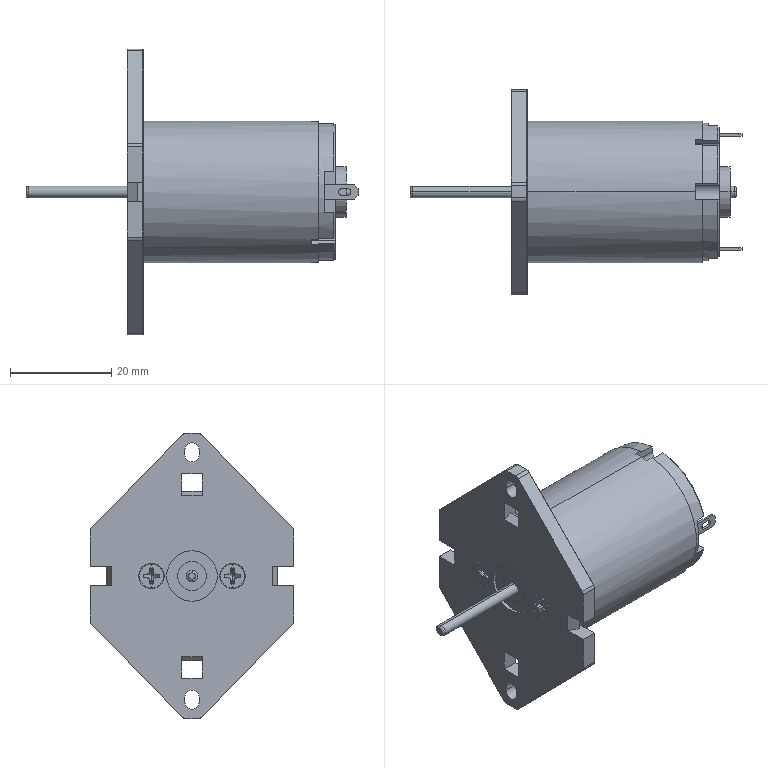Part | SolidWorks | features BaseBody 3 | 3 solids | 349 faces | box 65.53 x 40.25 x 56.3 mm | volume 27428 mm3 | cylinder 148 | plane 137 | cone 42 | torus 18 | spline 4 | commonest cylinder face diameters 0.2 x28 2.515 x26 1.799 x24 2.4 x16 2 x8 1.5 x4